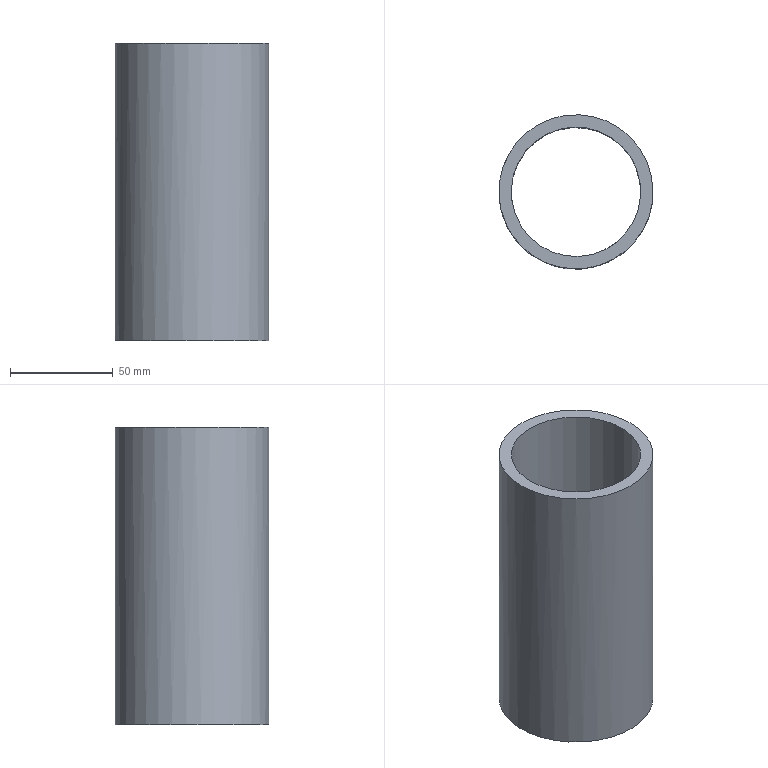Part | STEP file | gslz 2016.10.28-10_id18_x_t | 1 solid | 8 faces | box 75 x 75 x 145 mm | volume 187894 mm3 | plane 6 | cylinder 2 | commonest cylinder face diameters 63 x1 75 x1
STEP:
#1=CARTESIAN_POINT('',(0.,0.,0.));
#2=DIRECTION('',(0.,0.,1.));
#3=DIRECTION('',(1.,0.,0.));
#4=AXIS2_PLACEMENT_3D('',#1,#2,#3);
#5=CARTESIAN_POINT('',(-664.983,-298.483,-95.));
#6=VERTEX_POINT('',#5);
#7=CARTESIAN_POINT('',(-691.5,-325.,-95.));
#8=DIRECTION('',(0.,0.,1.));
#9=DIRECTION('',(0.7071,0.7071,0.));
#10=AXIS2_PLACEMENT_3D('',#7,#8,#9);
#11=CIRCLE('',#10,37.5);
#12=CARTESIAN_POINT('',(-691.5,-325.,-95.));
#13=DIRECTION('',(0.,0.,-1.));
#14=DIRECTION('',(0.7071,0.7071,0.));
#15=AXIS2_PLACEMENT_3D('',#12,#13,#14);
#16=PLANE('',#15);
#17=CARTESIAN_POINT('',(37.5,0.));
#18=CARTESIAN_POINT('',(37.5,-64.952));
#19=CARTESIAN_POINT('',(-18.75,-32.476));
#20=CARTESIAN_POINT('',(-75.,0.));
#21=CARTESIAN_POINT('',(-18.75,32.476));
#22=CARTESIAN_POINT('',(37.5,64.952));
#23=CARTESIAN_POINT('',(37.5,0.));
#24=(BOUNDED_CURVE()B_SPLINE_CURVE(2,(#17,#18,#19,#20,#21,#22,#23),.UNSPECIFIED.,.T.,.F.)B_SPLINE_CURVE_WITH_KNOTS((1,2,2,2,2,1),(-2.094,0.,2.094,4.189,6.283,8.378),.UNSPECIFIED.)CURVE()GEOMETRIC_REPRESENTATION_ITEM()RATIONAL_B_SPLINE_CURVE((1.,0.5,1.,0.5,1.,0.5,1.))REPRESENTATION_ITEM(''));
#25=(GEOMETRIC_REPRESENTATION_CONTEXT(2)PARAMETRIC_REPRESENTATION_CONTEXT()REPRESENTATION_CONTEXT('',''));
#26=DEFINITIONAL_REPRESENTATION('',(#24),#25);
#27=PCURVE('',#16,#26);
#28=CARTESIAN_POINT('',(-691.5,-325.,85.));
#29=DIRECTION('',(0.,0.,-1.));
#30=DIRECTION('',(0.7071,0.7071,0.));
#31=AXIS2_PLACEMENT_3D('',#28,#29,#30);
#32=CYLINDRICAL_SURFACE('',#31,37.5);
#33=CARTESIAN_POINT('',(6.283,180.));
#34=DIRECTION('',(-1.,0.));
#35=VECTOR('',#34,1.);
#36=LINE('',#33,#35);
#37=(GEOMETRIC_REPRESENTATION_CONTEXT(2)PARAMETRIC_REPRESENTATION_CONTEXT()REPRESENTATION_CONTEXT('',''));
#38=DEFINITIONAL_REPRESENTATION('',(#36),#37);
#39=PCURVE('',#32,#38);
#40=SURFACE_CURVE('',#11,(#27,#39),.PCURVE_S1.);
#41=EDGE_CURVE('',#6,#6,#40,.T.);
#42=ORIENTED_EDGE('',*,*,#41,.F.);
#43=EDGE_LOOP('',(#42));
#44=FACE_BOUND('',#43,.T.);
#45=CARTESIAN_POINT('',(-670.312,-348.309,-95.));
#46=VERTEX_POINT('',#45);
#47=CARTESIAN_POINT('',(-667.206,-345.051,-95.));
#48=VERTEX_POINT('',#47);
#49=CARTESIAN_POINT('',(-691.5,-325.,-95.));
#50=DIRECTION('',(0.,0.,-1.));
#51=DIRECTION('',(-0.7071,-0.7071,0.));
#52=AXIS2_PLACEMENT_3D('',#49,#50,#51);
#53=CIRCLE('',#52,31.5);
#54=CARTESIAN_POINT('',(0.,0.));
#55=DIRECTION('',(-1.,0.));
#56=AXIS2_PLACEMENT_2D('',#54,#55);
#57=CIRCLE('',#56,31.5);
#58=(GEOMETRIC_REPRESENTATION_CONTEXT(2)PARAMETRIC_REPRESENTATION_CONTEXT()REPRESENTATION_CONTEXT('',''));
#59=DEFINITIONAL_REPRESENTATION('',(#57),#58);
#60=PCURVE('',#16,#59);
#61=CARTESIAN_POINT('',(-691.5,-325.,85.));
#62=DIRECTION('',(0.,0.,-1.));
#63=DIRECTION('',(0.7071,0.7071,0.));
#64=AXIS2_PLACEMENT_3D('',#61,#62,#63);
#65=CYLINDRICAL_SURFACE('',#64,31.5);
#66=CARTESIAN_POINT('',(-3.142,180.));
#67=DIRECTION('',(1.,0.));
#68=VECTOR('',#67,1.);
#69=LINE('',#66,#68);
#70=(GEOMETRIC_REPRESENTATION_CONTEXT(2)PARAMETRIC_REPRESENTATION_CONTEXT()REPRESENTATION_CONTEXT('',''));
#71=DEFINITIONAL_REPRESENTATION('',(#69),#70);
#72=PCURVE('',#65,#71);
#73=SURFACE_CURVE('',#53,(#60,#72),.PCURVE_S1.);
#74=EDGE_CURVE('',#46,#48,#73,.T.);
#75=ORIENTED_EDGE('',*,*,#74,.F.);
#76=CARTESIAN_POINT('',(-668.873,-349.749,-95.));
#77=VERTEX_POINT('',#76);
#78=CARTESIAN_POINT('',(-673.822,-344.799,-95.));
#79=DIRECTION('',(0.7071,-0.7071,0.));
#80=VECTOR('',#79,1.);
#81=LINE('',#78,#80);
#82=CARTESIAN_POINT('',(-1.5,26.5));
#83=DIRECTION('',(0.,1.));
#84=VECTOR('',#83,1.);
#85=LINE('',#82,#84);
#86=(GEOMETRIC_REPRESENTATION_CONTEXT(2)PARAMETRIC_REPRESENTATION_CONTEXT()REPRESENTATION_CONTEXT('',''));
#87=DEFINITIONAL_REPRESENTATION('',(#85),#86);
#88=PCURVE('',#16,#87);
#89=CARTESIAN_POINT('',(-673.822,-344.799,1.));
#90=DIRECTION('',(0.7071,0.7071,0.));
#91=DIRECTION('',(0.,0.,1.));
#92=AXIS2_PLACEMENT_3D('',#89,#90,#91);
#93=PLANE('',#92);
#94=CARTESIAN_POINT('',(-96.,0.));
#95=DIRECTION('',(0.,1.));
#96=VECTOR('',#95,1.);
#97=LINE('',#94,#96);
#98=(GEOMETRIC_REPRESENTATION_CONTEXT(2)PARAMETRIC_REPRESENTATION_CONTEXT()REPRESENTATION_CONTEXT('',''));
#99=DEFINITIONAL_REPRESENTATION('',(#97),#98);
#100=PCURVE('',#93,#99);
#101=SURFACE_CURVE('',#81,(#88,#100),.PCURVE_S1.);
#102=EDGE_CURVE('',#46,#77,#101,.T.);
#103=ORIENTED_EDGE('',*,*,#102,.T.);
#104=CARTESIAN_POINT('',(-665.691,-346.567,-95.));
#105=VERTEX_POINT('',#104);
#106=CARTESIAN_POINT('',(-668.873,-349.749,-95.));
#107=DIRECTION('',(0.7071,0.7071,0.));
#108=VECTOR('',#107,1.);
#109=LINE('',#106,#108);
#110=CARTESIAN_POINT('',(-1.5,33.5));
#111=DIRECTION('',(1.,0.));
#112=VECTOR('',#111,1.);
#113=LINE('',#110,#112);
#114=(GEOMETRIC_REPRESENTATION_CONTEXT(2)PARAMETRIC_REPRESENTATION_CONTEXT()REPRESENTATION_CONTEXT('',''));
#115=DEFINITIONAL_REPRESENTATION('',(#113),#114);
#116=PCURVE('',#16,#115);
#117=CARTESIAN_POINT('',(-668.873,-349.749,1.));
#118=DIRECTION('',(-0.7071,0.7071,0.));
#119=DIRECTION('',(0.,0.,-1.));
#120=AXIS2_PLACEMENT_3D('',#117,#118,#119);
#121=PLANE('',#120);
#122=CARTESIAN_POINT('',(96.,0.));
#123=DIRECTION('',(0.,-1.));
#124=VECTOR('',#123,1.);
#125=LINE('',#122,#124);
#126=(GEOMETRIC_REPRESENTATION_CONTEXT(2)PARAMETRIC_REPRESENTATION_CONTEXT()REPRESENTATION_CONTEXT('',''));
#127=DEFINITIONAL_REPRESENTATION('',(#125),#126);
#128=PCURVE('',#121,#127);
#129=SURFACE_CURVE('',#109,(#116,#128),.PCURVE_S1.);
#130=EDGE_CURVE('',#77,#105,#129,.T.);
#131=ORIENTED_EDGE('',*,*,#130,.T.);
#132=CARTESIAN_POINT('',(-665.691,-346.567,-95.));
#133=DIRECTION('',(-0.7071,0.7071,0.));
#134=VECTOR('',#133,1.);
#135=LINE('',#132,#134);
#136=CARTESIAN_POINT('',(3.,33.5));
#137=DIRECTION('',(0.,-1.));
#138=VECTOR('',#137,1.);
#139=LINE('',#136,#138);
#140=(GEOMETRIC_REPRESENTATION_CONTEXT(2)PARAMETRIC_REPRESENTATION_CONTEXT()REPRESENTATION_CONTEXT('',''));
#141=DEFINITIONAL_REPRESENTATION('',(#139),#140);
#142=PCURVE('',#16,#141);
#143=CARTESIAN_POINT('',(-665.691,-346.567,1.));
#144=DIRECTION('',(-0.7071,-0.7071,0.));
#145=DIRECTION('',(0.,0.,-1.));
#146=AXIS2_PLACEMENT_3D('',#143,#144,#145);
#147=PLANE('',#146);
#148=CARTESIAN_POINT('',(96.,0.));
#149=DIRECTION('',(0.,-1.));
#150=VECTOR('',#149,1.);
#151=LINE('',#148,#150);
#152=(GEOMETRIC_REPRESENTATION_CONTEXT(2)PARAMETRIC_REPRESENTATION_CONTEXT()REPRESENTATION_CONTEXT('',''));
#153=DEFINITIONAL_REPRESENTATION('',(#151),#152);
#154=PCURVE('',#147,#153);
#155=SURFACE_CURVE('',#135,(#142,#154),.PCURVE_S1.);
#156=EDGE_CURVE('',#105,#48,#155,.T.);
#157=ORIENTED_EDGE('',*,*,#156,.T.);
#158=EDGE_LOOP('',(#75,#103,#131,#157));
#159=FACE_BOUND('',#158,.T.);
#160=ADVANCED_FACE('',(#44,#159),#16,.T.);
#161=CARTESIAN_POINT('',(-713.774,-347.274,50.));
#162=VERTEX_POINT('',#161);
#163=CARTESIAN_POINT('',(-667.206,-345.051,50.));
#164=VERTEX_POINT('',#163);
#165=CARTESIAN_POINT('',(-691.5,-325.,50.));
#166=DIRECTION('',(0.,0.,-1.));
#167=DIRECTION('',(-0.7071,-0.7071,0.));
#168=AXIS2_PLACEMENT_3D('',#165,#166,#167);
#169=CIRCLE('',#168,31.5);
#170=CARTESIAN_POINT('',(3.142,35.));
#171=DIRECTION('',(1.,0.));
#172=VECTOR('',#171,1.);
#173=LINE('',#170,#172);
#174=(GEOMETRIC_REPRESENTATION_CONTEXT(2)PARAMETRIC_REPRESENTATION_CONTEXT()REPRESENTATION_CONTEXT('',''));
#175=DEFINITIONAL_REPRESENTATION('',(#173),#174);
#176=PCURVE('',#65,#175);
#177=CARTESIAN_POINT('',(-691.5,-325.,50.));
#178=DIRECTION('',(0.,0.,1.));
#179=DIRECTION('',(-0.7071,-0.7071,0.));
#180=AXIS2_PLACEMENT_3D('',#177,#178,#179);
#181=PLANE('',#180);
#182=CARTESIAN_POINT('',(31.5,0.));
#183=CARTESIAN_POINT('',(31.5,-54.56));
#184=CARTESIAN_POINT('',(-15.75,-27.28));
#185=CARTESIAN_POINT('',(-63.,0.));
#186=CARTESIAN_POINT('',(-15.75,27.28));
#187=CARTESIAN_POINT('',(31.5,54.56));
#188=CARTESIAN_POINT('',(31.5,0.));
#189=(BOUNDED_CURVE()B_SPLINE_CURVE(2,(#182,#183,#184,#185,#186,#187,#188),.UNSPECIFIED.,.T.,.F.)B_SPLINE_CURVE_WITH_KNOTS((1,2,2,2,2,1),(-2.094,0.,2.094,4.189,6.283,8.378),.UNSPECIFIED.)CURVE()GEOMETRIC_REPRESENTATION_ITEM()RATIONAL_B_SPLINE_CURVE((1.,0.5,1.,0.5,1.,0.5,1.))REPRESENTATION_ITEM(''));
#190=(GEOMETRIC_REPRESENTATION_CONTEXT(2)PARAMETRIC_REPRESENTATION_CONTEXT()REPRESENTATION_CONTEXT('',''));
#191=DEFINITIONAL_REPRESENTATION('',(#189),#190);
#192=PCURVE('',#181,#191);
#193=SURFACE_CURVE('',#169,(#176,#192),.PCURVE_S1.);
#194=EDGE_CURVE('',#162,#164,#193,.T.);
#195=ORIENTED_EDGE('',*,*,#194,.T.);
#196=CARTESIAN_POINT('',(-667.206,-345.051,-19.));
#197=VERTEX_POINT('',#196);
#198=CARTESIAN_POINT('',(-667.206,-345.051,50.));
#199=CARTESIAN_POINT('',(-667.206,-345.051,-19.));
#200=B_SPLINE_CURVE_WITH_KNOTS('',1,(#198,#199),.UNSPECIFIED.,.F.,.F.,(2,2),(35.,104.),.PIECEWISE_BEZIER_KNOTS.);
#201=CARTESIAN_POINT('',(7.759,0.));
#202=DIRECTION('',(0.,1.));
#203=VECTOR('',#202,1.);
#204=LINE('',#201,#203);
#205=(GEOMETRIC_REPRESENTATION_CONTEXT(2)PARAMETRIC_REPRESENTATION_CONTEXT()REPRESENTATION_CONTEXT('',''));
#206=DEFINITIONAL_REPRESENTATION('',(#204),#205);
#207=PCURVE('',#65,#206);
#208=CARTESIAN_POINT('',(1.475,0.));
#209=DIRECTION('',(0.,1.));
#210=VECTOR('',#209,1.);
#211=LINE('',#208,#210);
#212=(GEOMETRIC_REPRESENTATION_CONTEXT(2)PARAMETRIC_REPRESENTATION_CONTEXT()REPRESENTATION_CONTEXT('',''));
#213=DEFINITIONAL_REPRESENTATION('',(#211),#212);
#214=PCURVE('',#65,#213);
#215=SEAM_CURVE('',#200,(#207,#214),.PCURVE_S1.);
#216=EDGE_CURVE('',#164,#197,#215,.T.);
#217=ORIENTED_EDGE('',*,*,#216,.T.);
#218=CARTESIAN_POINT('',(-667.206,-345.051,85.));
#219=DIRECTION('',(0.,0.,-1.));
#220=VECTOR('',#219,1.);
#221=LINE('',#218,#220);
#222=CARTESIAN_POINT('',(7.759,0.));
#223=DIRECTION('',(0.,1.));
#224=VECTOR('',#223,1.);
#225=LINE('',#222,#224);
#226=(GEOMETRIC_REPRESENTATION_CONTEXT(2)PARAMETRIC_REPRESENTATION_CONTEXT()REPRESENTATION_CONTEXT('',''));
#227=DEFINITIONAL_REPRESENTATION('',(#225),#226);
#228=PCURVE('',#65,#227);
#229=CARTESIAN_POINT('',(-84.,-2.143));
#230=DIRECTION('',(1.,0.));
#231=VECTOR('',#230,1.);
#232=LINE('',#229,#231);
#233=(GEOMETRIC_REPRESENTATION_CONTEXT(2)PARAMETRIC_REPRESENTATION_CONTEXT()REPRESENTATION_CONTEXT('',''));
#234=DEFINITIONAL_REPRESENTATION('',(#232),#233);
#235=PCURVE('',#147,#234);
#236=SURFACE_CURVE('',#221,(#228,#235),.PCURVE_S1.);
#237=EDGE_CURVE('',#197,#48,#236,.T.);
#238=ORIENTED_EDGE('',*,*,#237,.T.);
#239=ORIENTED_EDGE('',*,*,#74,.F.);
#240=CARTESIAN_POINT('',(-670.312,-348.309,-19.));
#241=VERTEX_POINT('',#240);
#242=CARTESIAN_POINT('',(-670.312,-348.309,85.));
#243=DIRECTION('',(0.,0.,1.));
#244=VECTOR('',#243,1.);
#245=LINE('',#242,#244);
#246=CARTESIAN_POINT('',(1.618,0.));
#247=DIRECTION('',(0.,-1.));
#248=VECTOR('',#247,1.);
#249=LINE('',#246,#248);
#250=(GEOMETRIC_REPRESENTATION_CONTEXT(2)PARAMETRIC_REPRESENTATION_CONTEXT()REPRESENTATION_CONTEXT('',''));
#251=DEFINITIONAL_REPRESENTATION('',(#249),#250);
#252=PCURVE('',#65,#251);
#253=CARTESIAN_POINT('',(84.,4.964));
#254=DIRECTION('',(1.,0.));
#255=VECTOR('',#254,1.);
#256=LINE('',#253,#255);
#257=(GEOMETRIC_REPRESENTATION_CONTEXT(2)PARAMETRIC_REPRESENTATION_CONTEXT()REPRESENTATION_CONTEXT('',''));
#258=DEFINITIONAL_REPRESENTATION('',(#256),#257);
#259=PCURVE('',#93,#258);
#260=SURFACE_CURVE('',#245,(#252,#259),.PCURVE_S1.);
#261=EDGE_CURVE('',#46,#241,#260,.T.);
#262=ORIENTED_EDGE('',*,*,#261,.T.);
#263=CARTESIAN_POINT('',(-691.5,-325.,-19.));
#264=DIRECTION('',(0.,0.,-1.));
#265=DIRECTION('',(0.7071,0.7071,0.));
#266=AXIS2_PLACEMENT_3D('',#263,#264,#265);
#267=CIRCLE('',#266,31.5);
#268=CARTESIAN_POINT('',(0.,104.));
#269=DIRECTION('',(1.,0.));
#270=VECTOR('',#269,1.);
#271=LINE('',#268,#270);
#272=(GEOMETRIC_REPRESENTATION_CONTEXT(2)PARAMETRIC_REPRESENTATION_CONTEXT()REPRESENTATION_CONTEXT('',''));
#273=DEFINITIONAL_REPRESENTATION('',(#271),#272);
#274=PCURVE('',#65,#273);
#275=CARTESIAN_POINT('',(-668.873,-349.749,-19.));
#276=DIRECTION('',(0.,0.,1.));
#277=DIRECTION('',(-0.7071,-0.7071,0.));
#278=AXIS2_PLACEMENT_3D('',#275,#276,#277);
#279=PLANE('',#278);
#280=CARTESIAN_POINT('',(-33.,-33.5));
#281=CARTESIAN_POINT('',(-33.,21.06));
#282=CARTESIAN_POINT('',(14.25,-6.22));
#283=CARTESIAN_POINT('',(61.5,-33.5));
#284=CARTESIAN_POINT('',(14.25,-60.78));
#285=CARTESIAN_POINT('',(-33.,-88.06));
#286=CARTESIAN_POINT('',(-33.,-33.5));
#287=(BOUNDED_CURVE()B_SPLINE_CURVE(2,(#280,#281,#282,#283,#284,#285,#286),.UNSPECIFIED.,.T.,.F.)B_SPLINE_CURVE_WITH_KNOTS((1,2,2,2,2,1),(-2.094,0.,2.094,4.189,6.283,8.378),.UNSPECIFIED.)CURVE()GEOMETRIC_REPRESENTATION_ITEM()RATIONAL_B_SPLINE_CURVE((1.,0.5,1.,0.5,1.,0.5,1.))REPRESENTATION_ITEM(''));
#288=(GEOMETRIC_REPRESENTATION_CONTEXT(2)PARAMETRIC_REPRESENTATION_CONTEXT()REPRESENTATION_CONTEXT('',''));
#289=DEFINITIONAL_REPRESENTATION('',(#287),#288);
#290=PCURVE('',#279,#289);
#291=SURFACE_CURVE('',#267,(#274,#290),.PCURVE_S1.);
#292=EDGE_CURVE('',#197,#241,#291,.T.);
#293=ORIENTED_EDGE('',*,*,#292,.F.);
#294=ORIENTED_EDGE('',*,*,#216,.F.);
#295=CARTESIAN_POINT('',(-691.5,-325.,50.));
#296=DIRECTION('',(0.,0.,-1.));
#297=DIRECTION('',(-0.7071,-0.7071,0.));
#298=AXIS2_PLACEMENT_3D('',#295,#296,#297);
#299=CIRCLE('',#298,31.5);
#300=CARTESIAN_POINT('',(-3.142,35.));
#301=DIRECTION('',(1.,0.));
#302=VECTOR('',#301,1.);
#303=LINE('',#300,#302);
#304=(GEOMETRIC_REPRESENTATION_CONTEXT(2)PARAMETRIC_REPRESENTATION_CONTEXT()REPRESENTATION_CONTEXT('',''));
#305=DEFINITIONAL_REPRESENTATION('',(#303),#304);
#306=PCURVE('',#65,#305);
#307=CARTESIAN_POINT('',(31.5,0.));
#308=CARTESIAN_POINT('',(31.5,-54.56));
#309=CARTESIAN_POINT('',(-15.75,-27.28));
#310=CARTESIAN_POINT('',(-63.,0.));
#311=CARTESIAN_POINT('',(-15.75,27.28));
#312=CARTESIAN_POINT('',(31.5,54.56));
#313=CARTESIAN_POINT('',(31.5,0.));
#314=(BOUNDED_CURVE()B_SPLINE_CURVE(2,(#307,#308,#309,#310,#311,#312,#313),.UNSPECIFIED.,.T.,.F.)B_SPLINE_CURVE_WITH_KNOTS((1,2,2,2,2,1),(-2.094,0.,2.094,4.189,6.283,8.378),.UNSPECIFIED.)CURVE()GEOMETRIC_REPRESENTATION_ITEM()RATIONAL_B_SPLINE_CURVE((1.,0.5,1.,0.5,1.,0.5,1.))REPRESENTATION_ITEM(''));
#315=(GEOMETRIC_REPRESENTATION_CONTEXT(2)PARAMETRIC_REPRESENTATION_CONTEXT()REPRESENTATION_CONTEXT('',''));
#316=DEFINITIONAL_REPRESENTATION('',(#314),#315);
#317=PCURVE('',#181,#316);
#318=SURFACE_CURVE('',#299,(#306,#317),.PCURVE_S1.);
#319=EDGE_CURVE('',#164,#162,#318,.T.);
#320=ORIENTED_EDGE('',*,*,#319,.T.);
#321=EDGE_LOOP('',(#195,#217,#238,#239,#262,#293,#294,#320));
#322=FACE_BOUND('',#321,.F.);
#323=ADVANCED_FACE('',(#322),#65,.F.);
#324=CARTESIAN_POINT('',(-718.017,-351.517,50.));
#325=VERTEX_POINT('',#324);
#326=CARTESIAN_POINT('',(-664.983,-298.483,50.));
#327=VERTEX_POINT('',#326);
#328=CARTESIAN_POINT('',(-691.5,-325.,50.));
#329=DIRECTION('',(0.,0.,-1.));
#330=DIRECTION('',(-0.7071,-0.7071,0.));
#331=AXIS2_PLACEMENT_3D('',#328,#329,#330);
#332=CIRCLE('',#331,37.5);
#333=CARTESIAN_POINT('',(3.142,35.));
#334=DIRECTION('',(1.,0.));
#335=VECTOR('',#334,1.);
#336=LINE('',#333,#335);
#337=(GEOMETRIC_REPRESENTATION_CONTEXT(2)PARAMETRIC_REPRESENTATION_CONTEXT()REPRESENTATION_CONTEXT('',''));
#338=DEFINITIONAL_REPRESENTATION('',(#336),#337);
#339=PCURVE('',#32,#338);
#340=CARTESIAN_POINT('',(37.5,0.));
#341=CARTESIAN_POINT('',(37.5,-64.952));
#342=CARTESIAN_POINT('',(-18.75,-32.476));
#343=CARTESIAN_POINT('',(-75.,0.));
#344=CARTESIAN_POINT('',(-18.75,32.476));
#345=CARTESIAN_POINT('',(37.5,64.952));
#346=CARTESIAN_POINT('',(37.5,0.));
#347=(BOUNDED_CURVE()B_SPLINE_CURVE(2,(#340,#341,#342,#343,#344,#345,#346),.UNSPECIFIED.,.T.,.F.)B_SPLINE_CURVE_WITH_KNOTS((1,2,2,2,2,1),(-2.094,0.,2.094,4.189,6.283,8.378),.UNSPECIFIED.)CURVE()GEOMETRIC_REPRESENTATION_ITEM()RATIONAL_B_SPLINE_CURVE((1.,0.5,1.,0.5,1.,0.5,1.))REPRESENTATION_ITEM(''));
#348=(GEOMETRIC_REPRESENTATION_CONTEXT(2)PARAMETRIC_REPRESENTATION_CONTEXT()REPRESENTATION_CONTEXT('',''));
#349=DEFINITIONAL_REPRESENTATION('',(#347),#348);
#350=PCURVE('',#181,#349);
#351=SURFACE_CURVE('',#332,(#339,#350),.PCURVE_S1.);
#352=EDGE_CURVE('',#325,#327,#351,.T.);
#353=ORIENTED_EDGE('',*,*,#352,.T.);
#354=CARTESIAN_POINT('',(-664.983,-298.483,50.));
#355=CARTESIAN_POINT('',(-664.983,-298.483,-95.));
#356=B_SPLINE_CURVE_WITH_KNOTS('',1,(#354,#355),.UNSPECIFIED.,.F.,.F.,(2,2),(35.,180.),.PIECEWISE_BEZIER_KNOTS.);
#357=CARTESIAN_POINT('',(6.283,0.));
#358=DIRECTION('',(0.,1.));
#359=VECTOR('',#358,1.);
#360=LINE('',#357,#359);
#361=(GEOMETRIC_REPRESENTATION_CONTEXT(2)PARAMETRIC_REPRESENTATION_CONTEXT()REPRESENTATION_CONTEXT('',''));
#362=DEFINITIONAL_REPRESENTATION('',(#360),#361);
#363=PCURVE('',#32,#362);
#364=CARTESIAN_POINT('',(0.,0.));
#365=DIRECTION('',(0.,1.));
#366=VECTOR('',#365,1.);
#367=LINE('',#364,#366);
#368=(GEOMETRIC_REPRESENTATION_CONTEXT(2)PARAMETRIC_REPRESENTATION_CONTEXT()REPRESENTATION_CONTEXT('',''));
#369=DEFINITIONAL_REPRESENTATION('',(#367),#368);
#370=PCURVE('',#32,#369);
#371=SEAM_CURVE('',#356,(#363,#370),.PCURVE_S1.);
#372=EDGE_CURVE('',#327,#6,#371,.T.);
#373=ORIENTED_EDGE('',*,*,#372,.T.);
#374=ORIENTED_EDGE('',*,*,#41,.T.);
#375=ORIENTED_EDGE('',*,*,#372,.F.);
#376=CARTESIAN_POINT('',(-691.5,-325.,50.));
#377=DIRECTION('',(0.,0.,-1.));
#378=DIRECTION('',(-0.7071,-0.7071,0.));
#379=AXIS2_PLACEMENT_3D('',#376,#377,#378);
#380=CIRCLE('',#379,37.5);
#381=CARTESIAN_POINT('',(-3.142,35.));
#382=DIRECTION('',(1.,0.));
#383=VECTOR('',#382,1.);
#384=LINE('',#381,#383);
#385=(GEOMETRIC_REPRESENTATION_CONTEXT(2)PARAMETRIC_REPRESENTATION_CONTEXT()REPRESENTATION_CONTEXT('',''));
#386=DEFINITIONAL_REPRESENTATION('',(#384),#385);
#387=PCURVE('',#32,#386);
#388=CARTESIAN_POINT('',(37.5,0.));
#389=CARTESIAN_POINT('',(37.5,-64.952));
#390=CARTESIAN_POINT('',(-18.75,-32.476));
#391=CARTESIAN_POINT('',(-75.,0.));
#392=CARTESIAN_POINT('',(-18.75,32.476));
#393=CARTESIAN_POINT('',(37.5,64.952));
#394=CARTESIAN_POINT('',(37.5,0.));
#395=(BOUNDED_CURVE()B_SPLINE_CURVE(2,(#388,#389,#390,#391,#392,#393,#394),.UNSPECIFIED.,.T.,.F.)B_SPLINE_CURVE_WITH_KNOTS((1,2,2,2,2,1),(-2.094,0.,2.094,4.189,6.283,8.378),.UNSPECIFIED.)CURVE()GEOMETRIC_REPRESENTATION_ITEM()RATIONAL_B_SPLINE_CURVE((1.,0.5,1.,0.5,1.,0.5,1.))REPRESENTATION_ITEM(''));
#396=(GEOMETRIC_REPRESENTATION_CONTEXT(2)PARAMETRIC_REPRESENTATION_CONTEXT()REPRESENTATION_CONTEXT('',''));
#397=DEFINITIONAL_REPRESENTATION('',(#395),#396);
#398=PCURVE('',#181,#397);
#399=SURFACE_CURVE('',#380,(#387,#398),.PCURVE_S1.);
#400=EDGE_CURVE('',#327,#325,#399,.T.);
#401=ORIENTED_EDGE('',*,*,#400,.T.);
#402=EDGE_LOOP('',(#353,#373,#374,#375,#401));
#403=FACE_BOUND('',#402,.T.);
#404=ADVANCED_FACE('',(#403),#32,.T.);
#405=ORIENTED_EDGE('',*,*,#194,.T.);
#406=ORIENTED_EDGE('',*,*,#319,.T.);
#407=EDGE_LOOP('',(#405,#406));
#408=FACE_BOUND('',#407,.T.);
#409=ORIENTED_EDGE('',*,*,#352,.F.);
#410=ORIENTED_EDGE('',*,*,#400,.F.);
#411=EDGE_LOOP('',(#409,#410));
#412=FACE_BOUND('',#411,.T.);
#413=ADVANCED_FACE('',(#408,#412),#181,.T.);
#414=ORIENTED_EDGE('',*,*,#261,.T.);
#415=CARTESIAN_POINT('',(-668.873,-349.749,-19.));
#416=VERTEX_POINT('',#415);
#417=CARTESIAN_POINT('',(-673.822,-344.799,-19.));
#418=DIRECTION('',(0.7071,-0.7071,0.));
#419=VECTOR('',#418,1.);
#420=LINE('',#417,#419);
#421=CARTESIAN_POINT('',(-20.,0.));
#422=DIRECTION('',(0.,1.));
#423=VECTOR('',#422,1.);
#424=LINE('',#421,#423);
#425=(GEOMETRIC_REPRESENTATION_CONTEXT(2)PARAMETRIC_REPRESENTATION_CONTEXT()REPRESENTATION_CONTEXT('',''));
#426=DEFINITIONAL_REPRESENTATION('',(#424),#425);
#427=PCURVE('',#93,#426);
#428=CARTESIAN_POINT('',(0.,-7.));
#429=DIRECTION('',(0.,1.));
#430=VECTOR('',#429,1.);
#431=LINE('',#428,#430);
#432=(GEOMETRIC_REPRESENTATION_CONTEXT(2)PARAMETRIC_REPRESENTATION_CONTEXT()REPRESENTATION_CONTEXT('',''));
#433=DEFINITIONAL_REPRESENTATION('',(#431),#432);
#434=PCURVE('',#279,#433);
#435=SURFACE_CURVE('',#420,(#427,#434),.PCURVE_S1.);
#436=EDGE_CURVE('',#241,#416,#435,.T.);
#437=ORIENTED_EDGE('',*,*,#436,.T.);
#438=CARTESIAN_POINT('',(-668.873,-349.749,1.));
#439=DIRECTION('',(0.,0.,-1.));
#440=VECTOR('',#439,1.);
#441=LINE('',#438,#440);
#442=CARTESIAN_POINT('',(0.,7.));
#443=DIRECTION('',(-1.,0.));
#444=VECTOR('',#443,1.);
#445=LINE('',#442,#444);
#446=(GEOMETRIC_REPRESENTATION_CONTEXT(2)PARAMETRIC_REPRESENTATION_CONTEXT()REPRESENTATION_CONTEXT('',''));
#447=DEFINITIONAL_REPRESENTATION('',(#445),#446);
#448=PCURVE('',#93,#447);
#449=CARTESIAN_POINT('',(0.,0.));
#450=DIRECTION('',(1.,0.));
#451=VECTOR('',#450,1.);
#452=LINE('',#449,#451);
#453=(GEOMETRIC_REPRESENTATION_CONTEXT(2)PARAMETRIC_REPRESENTATION_CONTEXT()REPRESENTATION_CONTEXT('',''));
#454=DEFINITIONAL_REPRESENTATION('',(#452),#453);
#455=PCURVE('',#121,#454);
#456=SURFACE_CURVE('',#441,(#448,#455),.PCURVE_S1.);
#457=EDGE_CURVE('',#416,#77,#456,.T.);
#458=ORIENTED_EDGE('',*,*,#457,.T.);
#459=ORIENTED_EDGE('',*,*,#102,.F.);
#460=EDGE_LOOP('',(#414,#437,#458,#459));
#461=FACE_BOUND('',#460,.T.);
#462=ADVANCED_FACE('',(#461),#93,.T.);
#463=ORIENTED_EDGE('',*,*,#237,.T.);
#464=ORIENTED_EDGE('',*,*,#156,.F.);
#465=CARTESIAN_POINT('',(-665.691,-346.567,-19.));
#466=VERTEX_POINT('',#465);
#467=CARTESIAN_POINT('',(-665.691,-346.567,1.));
#468=DIRECTION('',(0.,0.,-1.));
#469=VECTOR('',#468,1.);
#470=LINE('',#467,#469);
#471=CARTESIAN_POINT('',(0.,0.));
#472=DIRECTION('',(1.,0.));
#473=VECTOR('',#472,1.);
#474=LINE('',#471,#473);
#475=(GEOMETRIC_REPRESENTATION_CONTEXT(2)PARAMETRIC_REPRESENTATION_CONTEXT()REPRESENTATION_CONTEXT('',''));
#476=DEFINITIONAL_REPRESENTATION('',(#474),#475);
#477=PCURVE('',#147,#476);
#478=CARTESIAN_POINT('',(0.,-4.5));
#479=DIRECTION('',(1.,0.));
#480=VECTOR('',#479,1.);
#481=LINE('',#478,#480);
#482=(GEOMETRIC_REPRESENTATION_CONTEXT(2)PARAMETRIC_REPRESENTATION_CONTEXT()REPRESENTATION_CONTEXT('',''));
#483=DEFINITIONAL_REPRESENTATION('',(#481),#482);
#484=PCURVE('',#121,#483);
#485=SURFACE_CURVE('',#470,(#477,#484),.PCURVE_S1.);
#486=EDGE_CURVE('',#466,#105,#485,.T.);
#487=ORIENTED_EDGE('',*,*,#486,.F.);
#488=CARTESIAN_POINT('',(-665.691,-346.567,-19.));
#489=DIRECTION('',(-0.7071,0.7071,0.));
#490=VECTOR('',#489,1.);
#491=LINE('',#488,#490);
#492=CARTESIAN_POINT('',(20.,0.));
#493=DIRECTION('',(0.,-1.));
#494=VECTOR('',#493,1.);
#495=LINE('',#492,#494);
#496=(GEOMETRIC_REPRESENTATION_CONTEXT(2)PARAMETRIC_REPRESENTATION_CONTEXT()REPRESENTATION_CONTEXT('',''));
#497=DEFINITIONAL_REPRESENTATION('',(#495),#496);
#498=PCURVE('',#147,#497);
#499=CARTESIAN_POINT('',(-4.5,0.));
#500=DIRECTION('',(0.,-1.));
#501=VECTOR('',#500,1.);
#502=LINE('',#499,#501);
#503=(GEOMETRIC_REPRESENTATION_CONTEXT(2)PARAMETRIC_REPRESENTATION_CONTEXT()REPRESENTATION_CONTEXT('',''));
#504=DEFINITIONAL_REPRESENTATION('',(#502),#503);
#505=PCURVE('',#279,#504);
#506=SURFACE_CURVE('',#491,(#498,#505),.PCURVE_S1.);
#507=EDGE_CURVE('',#466,#197,#506,.T.);
#508=ORIENTED_EDGE('',*,*,#507,.T.);
#509=EDGE_LOOP('',(#463,#464,#487,#508));
#510=FACE_BOUND('',#509,.T.);
#511=ADVANCED_FACE('',(#510),#147,.T.);
#512=ORIENTED_EDGE('',*,*,#507,.F.);
#513=CARTESIAN_POINT('',(-668.873,-349.749,-19.));
#514=DIRECTION('',(0.7071,0.7071,0.));
#515=VECTOR('',#514,1.);
#516=LINE('',#513,#515);
#517=CARTESIAN_POINT('',(0.,0.));
#518=DIRECTION('',(-1.,0.));
#519=VECTOR('',#518,1.);
#520=LINE('',#517,#519);
#521=(GEOMETRIC_REPRESENTATION_CONTEXT(2)PARAMETRIC_REPRESENTATION_CONTEXT()REPRESENTATION_CONTEXT('',''));
#522=DEFINITIONAL_REPRESENTATION('',(#520),#521);
#523=PCURVE('',#279,#522);
#524=CARTESIAN_POINT('',(20.,0.));
#525=DIRECTION('',(0.,-1.));
#526=VECTOR('',#525,1.);
#527=LINE('',#524,#526);
#528=(GEOMETRIC_REPRESENTATION_CONTEXT(2)PARAMETRIC_REPRESENTATION_CONTEXT()REPRESENTATION_CONTEXT('',''));
#529=DEFINITIONAL_REPRESENTATION('',(#527),#528);
#530=PCURVE('',#121,#529);
#531=SURFACE_CURVE('',#516,(#523,#530),.PCURVE_S1.);
#532=EDGE_CURVE('',#416,#466,#531,.T.);
#533=ORIENTED_EDGE('',*,*,#532,.F.);
#534=ORIENTED_EDGE('',*,*,#436,.F.);
#535=ORIENTED_EDGE('',*,*,#292,.F.);
#536=EDGE_LOOP('',(#512,#533,#534,#535));
#537=FACE_BOUND('',#536,.T.);
#538=ADVANCED_FACE('',(#537),#279,.F.);
#539=ORIENTED_EDGE('',*,*,#130,.F.);
#540=ORIENTED_EDGE('',*,*,#457,.F.);
#541=ORIENTED_EDGE('',*,*,#532,.T.);
#542=ORIENTED_EDGE('',*,*,#486,.T.);
#543=EDGE_LOOP('',(#539,#540,#541,#542));
#544=FACE_BOUND('',#543,.T.);
#545=ADVANCED_FACE('',(#544),#121,.T.);
#546=CLOSED_SHELL('',(#160,#323,#404,#413,#462,#511,#538,#545));
#547=MANIFOLD_SOLID_BREP('',#546);
#548=(LENGTH_UNIT()NAMED_UNIT(*)SI_UNIT(.MILLI.,.METRE.));
#549=UNCERTAINTY_MEASURE_WITH_UNIT(LENGTH_MEASURE(0.000002),#548,'','');
#550=(NAMED_UNIT(*)PLANE_ANGLE_UNIT()SI_UNIT($,.RADIAN.));
#551=(NAMED_UNIT(*)SI_UNIT($,.STERADIAN.)SOLID_ANGLE_UNIT());
#552=(GEOMETRIC_REPRESENTATION_CONTEXT(3)GLOBAL_UNCERTAINTY_ASSIGNED_CONTEXT((#549))GLOBAL_UNIT_ASSIGNED_CONTEXT((#548,#550,#551))REPRESENTATION_CONTEXT('',''));
#553=ADVANCED_BREP_SHAPE_REPRESENTATION('',(#4,#547),#552);